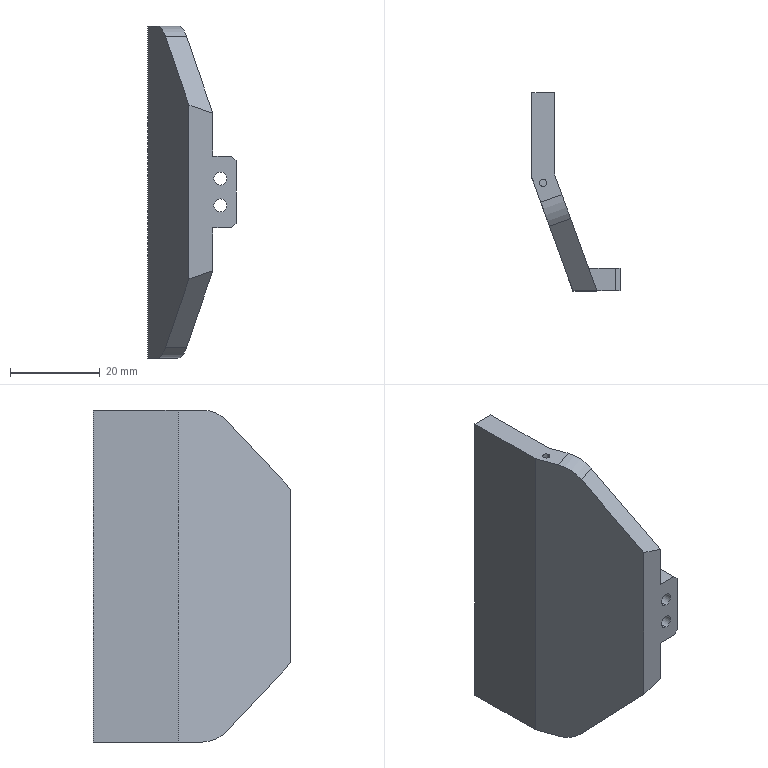CAM job | NX | 3+2 milling, 5-axis milling, drilling | part box 19.643 x 44.061 x 74 mm | stock box 25.643 x 65 x 79.357 mm
Tools:
number,name,description,diameter,corner_radius,flute_length,length,flutes
5,D4点钻,定心钻D4,4.0,0.0,43.0,75.0,2
11,D3开粗,D3,3.0,0.0,9.0,50.0,2
2,D8开粗,D8,8.0,0.0,25.0,60.0,2
3,D8精光,D8,8.0,0.0,20.0,60.0,2
4,R1,球头铣刀,2.0,1.0,4.0,4.0,2
6,D2.3钻头,Drilling Tool,2.3,0.0,35.0,50.0,2
7,M2.5丝攻,Drilling Tool,2.5,0.0,35.0,50.0,2
8,D2.9钻头,Drilling Tool,2.9,0.0,35.0,50.0,2
9,D1.8钻头,Drilling Tool,1.8,0.0,35.0,50.0,2
10,M2丝攻,Drilling Tool,2.0,0.0,35.0,50.0,2
Operations:
program,operation,operation_type,tool,method,geometry_group,spindle_rpm,surface_speed,feed_per_tooth,feed_cut,feed_plunge,cut_length_mm,path_length_mm,cut_time_min,machine_time_min
G54,ADAPTIVE_MILLING_1,CavityMilling,D8开粗,METHOD,W-G54,6500.0,100.0,0.1178,3000.0,100.0,10809.969,16682.828,2.776,3.363
G54,FLOOR_FACING,VolumeBased25DMillingOperation,D8精光,METHOD,MCS_G54,5500.0,138.0,0.0727,800.0,100.0,267.058,352.345,0.3338,0.3424
G54,FLOOR_FACING_COPY,VolumeBased25DMillingOperation,D8精光,METHOD,MCS_G54,5500.0,138.0,0.0727,800.0,100.0,30.0,86.0,0.0375,0.0431
G54,PLANAR_MILL_6_COPY,PlanarMilling,D8精光,METHOD,MCS_G54,4500.0,113.0,0.0889,800.0,100.0,56.0,220.0,0.07,0.0864
G54,PLANAR_MILL_6,PlanarMilling,D8精光,METHOD,MCS_G54,4500.0,113.0,0.0889,800.0,100.0,304.775,586.775,0.381,0.4092
G54,CURVE_DRIVE_1,SurfaceContour,R1,METHOD,MCS_G54,4500.0,100.0,0.1178,1000.0,100.0,488.829,614.722,0.4888,0.5014
G55,FLOOR_FACING_1_COPY,VolumeBased25DMillingOperation,D8开粗,METHOD,W-G55,5500.0,100.0,0.1178,800.0,100.0,356.92,410.72,0.4462,0.4515
G55,PLANAR_MILL_4_COPY_1,PlanarMilling,D8开粗,METHOD,W-G55,5500.0,100.0,0.1178,800.0,100.0,61.522,115.322,0.0769,0.0823
G55,FLOOR_FACING_1,VolumeBased25DMillingOperation,D8精光,METHOD,W-G55,5500.0,100.0,0.1178,800.0,100.0,354.145,408.145,0.4427,0.4481
G55,PLANAR_MILL_4,PlanarMilling,D8精光,METHOD,W-G55,5500.0,100.0,0.1178,800.0,100.0,61.208,115.208,0.0765,0.0819
G55,PLANAR_MILL_4_COPY,PlanarMilling,D8精光,METHOD,W-G55,5500.0,100.0,0.1178,800.0,100.0,96.0,150.0,0.12,0.1254
G55,PLANAR_MILL_4_COPY_COPY,PlanarMilling,D8精光,METHOD,W-G55,5500.0,100.0,0.1178,800.0,100.0,175.563,572.134,0.2195,0.2591
G55,3_AXIS_DEBURRING_1,TpMultiAxisDeburring,R1,METHOD,MCS_G55,4500.0,0.0,0.0,600.0,90.0,237.953,363.646,0.3979,0.3979
G56,DRILLING_1,Operation,D4点钻,METHOD,MCS_G56,3000.0,0.0,0.0,200.0,0.0,6.9,62.125,0.0345,0.04
G56,DRILLING_1_COPY,Operation,D2.9钻头,METHOD,MCS_G56,3000.0,0.0,0.0,200.0,0.0,18.0,84.325,0.09,0.0966
G57,ADAPTIVE_MILLING,CavityMilling,D8开粗,METHOD,W57,6500.0,100.0,0.1178,2500.0,100.0,11358.841,12964.919,4.453,4.614
G57,FLOOR_FACING_2,VolumeBased25DMillingOperation,D8精光,METHOD,MCS_G57,4500.0,113.0,0.0889,800.0,100.0,355.943,409.943,0.4449,0.4503
G58,FLOOR_FACING_3,VolumeBased25DMillingOperation,D8开粗,METHOD,MCS_G58,4500.0,113.0,0.0889,800.0,100.0,404.568,458.368,0.5057,0.5111
G58,FLOOR_FACING_3_COPY,VolumeBased25DMillingOperation,D8精光,METHOD,MCS_G58,4500.0,113.0,0.0889,800.0,100.0,404.568,458.568,0.5057,0.5111
G58,PLANAR_MILL,PlanarMilling,D8开粗,METHOD,MCS_G58,4500.0,113.0,0.2222,2000.0,100.0,7317.566,7384.566,3.659,3.666
G58,PLANAR_MILL_COPY,PlanarMilling,D8精光,METHOD,MCS_G58,4500.0,113.0,0.0667,600.0,100.0,331.406,405.406,0.5523,0.5597
G58,PLANAR_MILL_COPY_COPY,PlanarMilling,D8精光,METHOD,MCS_G58,4500.0,113.0,0.0667,600.0,100.0,331.892,405.892,0.5532,0.5606
G58,CURVE_DRIVE,SurfaceContour,R1,METHOD,MCS_G58,6500.0,100.0,0.1178,2500.0,100.0,1909.39,1963.397,0.7638,0.7692
G58,3_AXIS_DEBURRING,TpMultiAxisDeburring,R1,METHOD,MCS_G58,4500.0,0.0,0.0,800.0,90.0,224.722,303.467,0.2814,0.2814
G58,3_AXIS_DEBURRING_1_COPY,TpMultiAxisDeburring,R1,METHOD,MCS_G58,4500.0,0.0,0.0,800.0,90.0,34.705,91.815,0.0436,0.0436
G59,PLANAR_MILL_1,PlanarMilling,D3开粗,METHOD,MCS_G57,4500.0,42.0,0.2222,2000.0,100.0,703.041,3041.302,0.3515,0.5853
G54.1,PLANAR_MILL_2,PlanarMilling,D8开粗,METHOD,MCS_G54.1,3500.0,87.0,0.1143,800.0,100.0,40.0,203.8,0.05,0.0664
G54.1,PLANAR_MILL_2_COPY_COPY,PlanarMilling,D8精光,METHOD,MCS_G54.1,3500.0,87.0,0.1143,800.0,100.0,40.0,204.0,0.05,0.0664
G54.1,PLANAR_MILL_3,PlanarMilling,D4点钻,METHOD,MCS_G54.1,3500.0,43.0,0.1143,800.0,100.0,56.0,367.1,0.07,0.1011
G54.1,PLANAR_MILL_3_COPY,PlanarMilling,D4点钻,METHOD,MCS_G54.1,4500.0,56.0,0.0667,600.0,100.0,56.0,367.0,0.0933,0.1244
G54.1,DRILLING,Operation,D4点钻,METHOD,MCS_G54.1,3000.0,0.0,0.0,200.0,0.0,8.6,148.266,0.043,0.057
G54.1,DRILLING_COPY,Operation,D2.3钻头,METHOD,MCS_G54.1,3000.0,0.0,0.0,150.0,0.0,20.0,171.066,0.1333,0.1484
G54.1,DRILLING_COPY_COPY,Operation,M2.5丝攻,METHOD,MCS_G54.1,300.0,2.0,0.0008,0.45,0.0,18.0,167.066,40.0,40.015
G54.2,SPOT_FACING,Operation,D4点钻,METHOD,MCS-G54.2,3000.0,0.0,0.0,200.0,0.0,3.0,66.0,0.015,0.0213
G54.2,SPOT_FACING_COPY,Operation,D1.8钻头,METHOD,MCS-G54.2,3000.0,16.0,0.025,150.0,0.0,10.0,80.0,0.0667,0.0737
G54.2,SPOT_FACING_COPY_COPY,Operation,M2丝攻,METHOD,MCS-G54.2,300.0,1.0,0.0007,0.4,0.0,9.0,78.0,22.5,22.507
G54.3,SPOT_FACING_1,Operation,D4点钻,METHOD,MCS_G54.3,3000.0,37.0,0.0333,200.0,0.0,7.0,74.0,0.035,0.0417
G54.3,SPOT_FACING_1_COPY,Operation,D1.8钻头,METHOD,MCS_G54.3,3000.0,16.0,0.025,150.0,0.0,14.0,88.0,0.0933,0.1007
G54.3,SPOT_FACING_1_COPY_COPY,Operation,M2丝攻,METHOD,MCS_G54.3,3000.0,18.0,0.0001,0.4,0.0,13.0,86.0,32.5,32.507